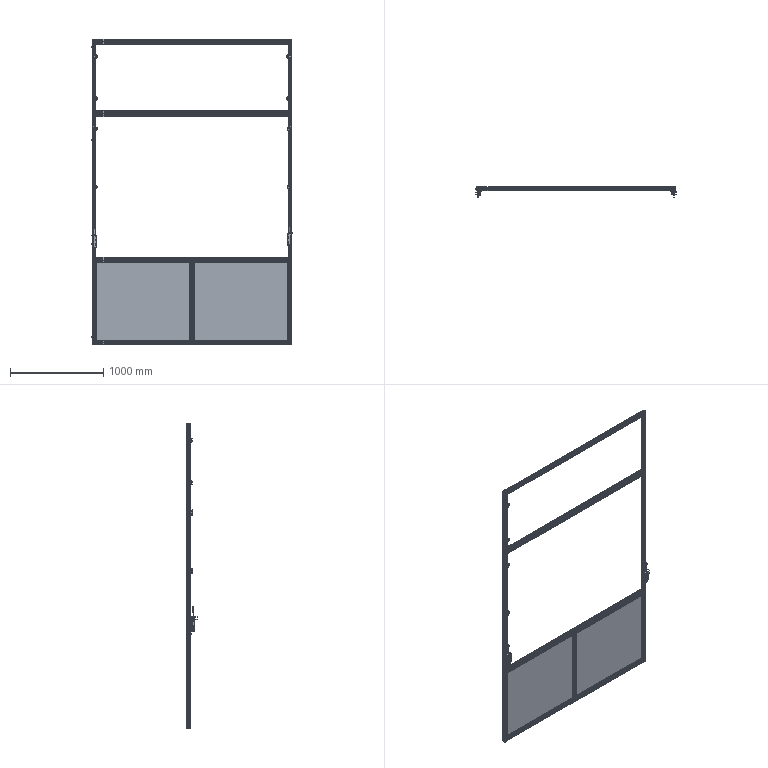Part | SolidWorks | features ReferencePattern 98, LocalLPattern 9 | 249 solids | 14268 faces | volume 20597906 mm3 | plane 7957 | cylinder 3744 | cone 1767 | spline 460 | torus 272 | sphere 68 | commonest cylinder face diameters 2.5 x336 1 x290 2 x286 5 x220 8 x220 0.562 x200